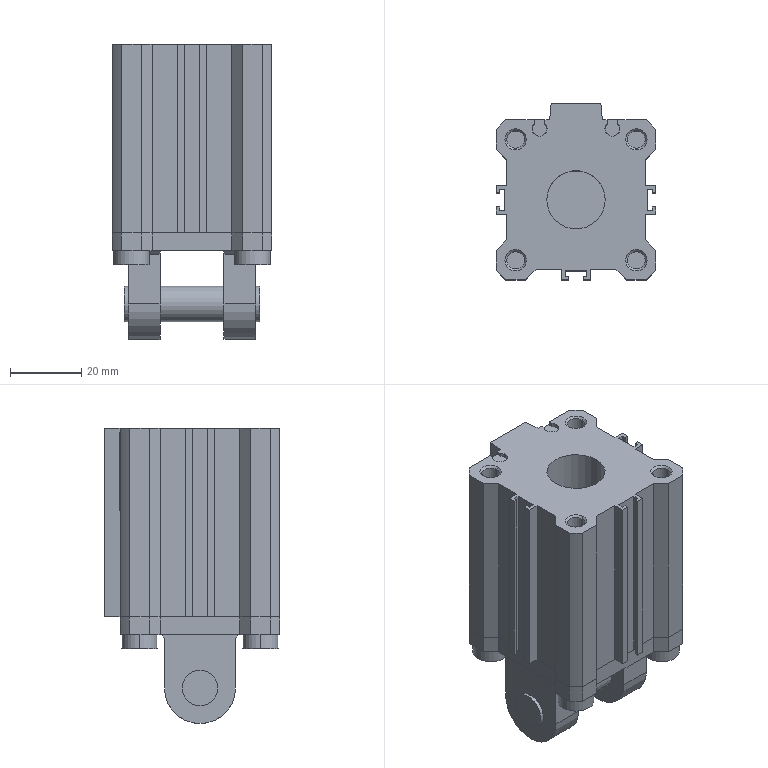Part | NX | features BREP 1 | 1 solid | 204 faces | box 45 x 49.5 x 83 mm | volume 105739 mm3 | plane 129 | cylinder 55 | cone 20 | commonest cylinder face diameters 10 x14 4.92 x8 4 x6 4.2 x6 2.7 x4 8.57 x4